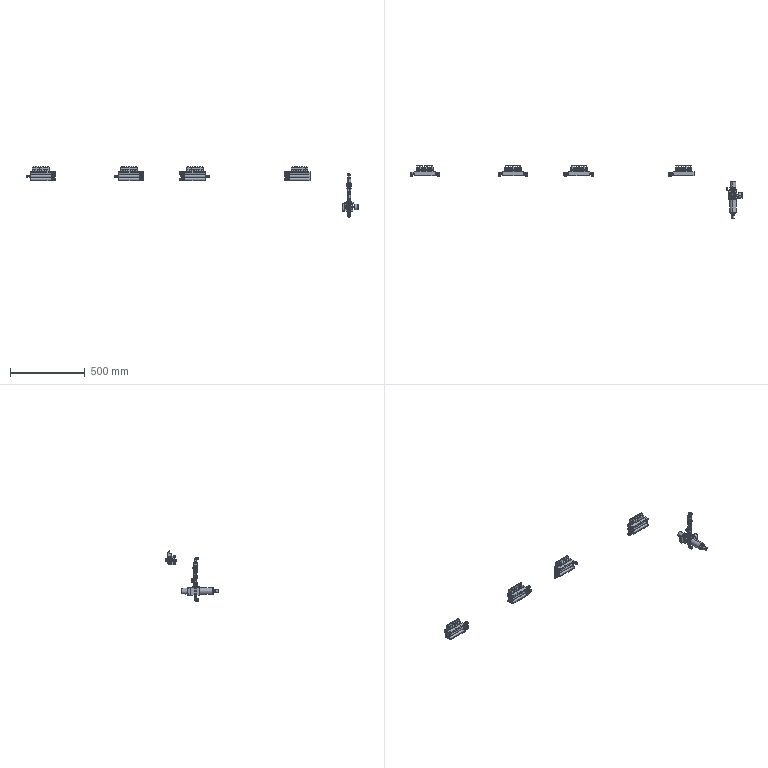Part | NX | 58 solids | 20112 faces | volume 2135104 mm3 | plane 16892 | cylinder 2474 | cone 649 | torus 66 | sphere 18 | spline 13 | commonest cylinder face diameters 2 x384 4 x346 9 x224 2.5 x168 7.938 x168 14 x140